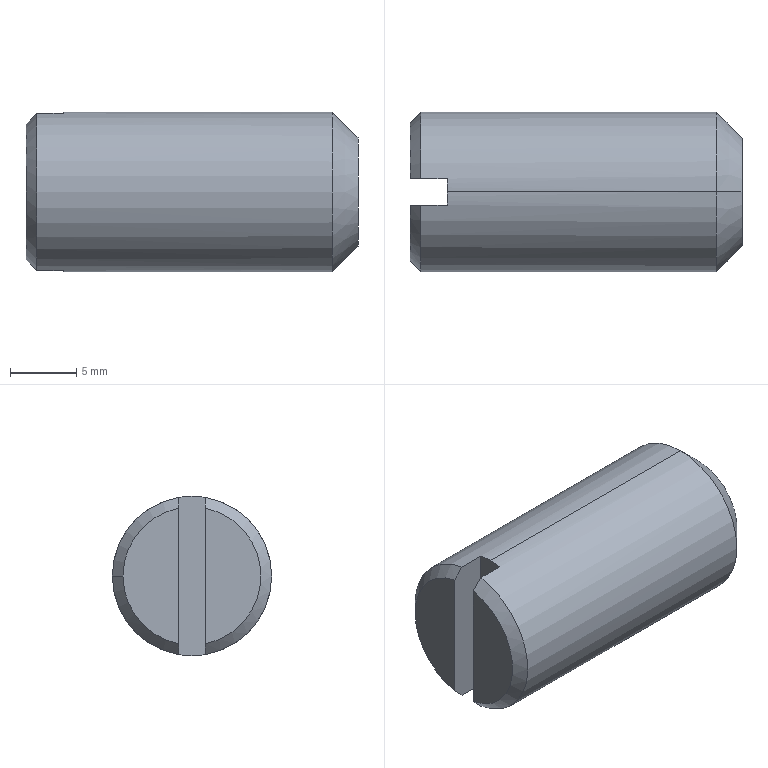Part | STEP file | 1 solid | 13 faces | box 25 x 12 x 12 mm | volume 2688 mm3 | plane 6 | cone 5 | cylinder 2 | commonest cylinder face diameters 12 x2
STEP:
#1=CARTESIAN_POINT('',(0.,0.,0.));
#2=DIRECTION('',(0.,0.,1.));
#3=DIRECTION('',(1.,0.,0.));
#4=AXIS2_PLACEMENT_3D('',#1,#2,#3);
#5=CARTESIAN_POINT('',(0.,-1.,5.099));
#6=VERTEX_POINT('',#5);
#7=CARTESIAN_POINT('',(0.,-1.,-5.099));
#8=VERTEX_POINT('',#7);
#9=CARTESIAN_POINT('',(0.,-1.,-50.));
#10=DIRECTION('',(0.,0.,-1.));
#11=VECTOR('',#10,1.);
#12=LINE('',#9,#11);
#13=CARTESIAN_POINT('',(0.,5.196,0.));
#14=DIRECTION('',(1.,0.,0.));
#15=DIRECTION('',(0.,1.,0.));
#16=AXIS2_PLACEMENT_3D('',#13,#14,#15);
#17=PLANE('',#16);
#18=CARTESIAN_POINT('',(-6.196,-50.));
#19=DIRECTION('',(0.,-1.));
#20=VECTOR('',#19,1.);
#21=LINE('',#18,#20);
#22=(GEOMETRIC_REPRESENTATION_CONTEXT(2)PARAMETRIC_REPRESENTATION_CONTEXT()REPRESENTATION_CONTEXT('',''));
#23=DEFINITIONAL_REPRESENTATION('',(#21),#22);
#24=PCURVE('',#17,#23);
#25=CARTESIAN_POINT('',(0.,-1.,-50.));
#26=DIRECTION('',(0.,-1.,0.));
#27=DIRECTION('',(0.,0.,-1.));
#28=AXIS2_PLACEMENT_3D('',#25,#26,#27);
#29=PLANE('',#28);
#30=CARTESIAN_POINT('',(0.,0.));
#31=DIRECTION('',(1.,0.));
#32=VECTOR('',#31,1.);
#33=LINE('',#30,#32);
#34=(GEOMETRIC_REPRESENTATION_CONTEXT(2)PARAMETRIC_REPRESENTATION_CONTEXT()REPRESENTATION_CONTEXT('',''));
#35=DEFINITIONAL_REPRESENTATION('',(#33),#34);
#36=PCURVE('',#29,#35);
#37=SURFACE_CURVE('',#12,(#24,#36),.PCURVE_S1.);
#38=EDGE_CURVE('',#6,#8,#37,.T.);
#39=ORIENTED_EDGE('',*,*,#38,.T.);
#40=CARTESIAN_POINT('',(0.,0.,0.));
#41=DIRECTION('',(1.,0.,0.));
#42=DIRECTION('',(0.,1.,0.));
#43=AXIS2_PLACEMENT_3D('',#40,#41,#42);
#44=CIRCLE('',#43,5.196);
#45=CARTESIAN_POINT('',(-5.196,0.));
#46=DIRECTION('',(1.,0.));
#47=AXIS2_PLACEMENT_2D('',#45,#46);
#48=CIRCLE('',#47,5.196);
#49=(GEOMETRIC_REPRESENTATION_CONTEXT(2)PARAMETRIC_REPRESENTATION_CONTEXT()REPRESENTATION_CONTEXT('',''));
#50=DEFINITIONAL_REPRESENTATION('',(#48),#49);
#51=PCURVE('',#17,#50);
#52=CARTESIAN_POINT('',(0.804,0.,0.));
#53=DIRECTION('',(1.,0.,0.));
#54=DIRECTION('',(0.,1.,0.));
#55=AXIS2_PLACEMENT_3D('',#52,#53,#54);
#56=CONICAL_SURFACE('',#55,6.,0.7854);
#57=CARTESIAN_POINT('',(0.,-0.804));
#58=DIRECTION('',(1.,0.));
#59=VECTOR('',#58,1.);
#60=LINE('',#57,#59);
#61=(GEOMETRIC_REPRESENTATION_CONTEXT(2)PARAMETRIC_REPRESENTATION_CONTEXT()REPRESENTATION_CONTEXT('',''));
#62=DEFINITIONAL_REPRESENTATION('',(#60),#61);
#63=PCURVE('',#56,#62);
#64=SURFACE_CURVE('',#44,(#51,#63),.PCURVE_S1.);
#65=EDGE_CURVE('',#6,#8,#64,.T.);
#66=ORIENTED_EDGE('',*,*,#65,.F.);
#67=EDGE_LOOP('',(#39,#66));
#68=FACE_BOUND('',#67,.T.);
#69=ADVANCED_FACE('',(#68),#17,.F.);
#70=CARTESIAN_POINT('',(25.,0.,4.07));
#71=VERTEX_POINT('',#70);
#72=CARTESIAN_POINT('',(25.,0.,-4.07));
#73=VERTEX_POINT('',#72);
#74=CARTESIAN_POINT('',(25.,0.,0.));
#75=DIRECTION('',(-1.,0.,0.));
#76=DIRECTION('',(0.,0.,1.));
#77=AXIS2_PLACEMENT_3D('',#74,#75,#76);
#78=CIRCLE('',#77,4.07);
#79=CARTESIAN_POINT('',(25.,0.,0.));
#80=DIRECTION('',(-1.,0.,0.));
#81=DIRECTION('',(0.,0.,1.));
#82=AXIS2_PLACEMENT_3D('',#79,#80,#81);
#83=PLANE('',#82);
#84=CARTESIAN_POINT('',(0.,0.));
#85=DIRECTION('',(1.,0.));
#86=AXIS2_PLACEMENT_2D('',#84,#85);
#87=CIRCLE('',#86,4.07);
#88=(GEOMETRIC_REPRESENTATION_CONTEXT(2)PARAMETRIC_REPRESENTATION_CONTEXT()REPRESENTATION_CONTEXT('',''));
#89=DEFINITIONAL_REPRESENTATION('',(#87),#88);
#90=PCURVE('',#83,#89);
#91=CARTESIAN_POINT('',(23.07,0.,0.));
#92=DIRECTION('',(-1.,0.,0.));
#93=DIRECTION('',(0.,0.,1.));
#94=AXIS2_PLACEMENT_3D('',#91,#92,#93);
#95=CONICAL_SURFACE('',#94,6.,0.7854);
#96=CARTESIAN_POINT('',(0.,-1.93));
#97=DIRECTION('',(1.,0.));
#98=VECTOR('',#97,1.);
#99=LINE('',#96,#98);
#100=(GEOMETRIC_REPRESENTATION_CONTEXT(2)PARAMETRIC_REPRESENTATION_CONTEXT()REPRESENTATION_CONTEXT('',''));
#101=DEFINITIONAL_REPRESENTATION('',(#99),#100);
#102=PCURVE('',#95,#101);
#103=SURFACE_CURVE('',#78,(#90,#102),.PCURVE_S1.);
#104=EDGE_CURVE('',#71,#73,#103,.T.);
#105=ORIENTED_EDGE('',*,*,#104,.F.);
#106=CARTESIAN_POINT('',(25.,0.,0.));
#107=DIRECTION('',(-1.,0.,0.));
#108=DIRECTION('',(0.,0.,1.));
#109=AXIS2_PLACEMENT_3D('',#106,#107,#108);
#110=CIRCLE('',#109,4.07);
#111=CARTESIAN_POINT('',(0.,0.));
#112=DIRECTION('',(1.,0.));
#113=AXIS2_PLACEMENT_2D('',#111,#112);
#114=CIRCLE('',#113,4.07);
#115=(GEOMETRIC_REPRESENTATION_CONTEXT(2)PARAMETRIC_REPRESENTATION_CONTEXT()REPRESENTATION_CONTEXT('',''));
#116=DEFINITIONAL_REPRESENTATION('',(#114),#115);
#117=PCURVE('',#83,#116);
#118=CARTESIAN_POINT('',(23.07,0.,0.));
#119=DIRECTION('',(-1.,0.,0.));
#120=DIRECTION('',(0.,0.,1.));
#121=AXIS2_PLACEMENT_3D('',#118,#119,#120);
#122=CONICAL_SURFACE('',#121,6.,0.7854);
#123=CARTESIAN_POINT('',(0.,-1.93));
#124=DIRECTION('',(1.,0.));
#125=VECTOR('',#124,1.);
#126=LINE('',#123,#125);
#127=(GEOMETRIC_REPRESENTATION_CONTEXT(2)PARAMETRIC_REPRESENTATION_CONTEXT()REPRESENTATION_CONTEXT('',''));
#128=DEFINITIONAL_REPRESENTATION('',(#126),#127);
#129=PCURVE('',#122,#128);
#130=SURFACE_CURVE('',#110,(#117,#129),.PCURVE_S1.);
#131=EDGE_CURVE('',#73,#71,#130,.T.);
#132=ORIENTED_EDGE('',*,*,#131,.F.);
#133=EDGE_LOOP('',(#105,#132));
#134=FACE_BOUND('',#133,.T.);
#135=ADVANCED_FACE('',(#134),#83,.F.);
#136=CARTESIAN_POINT('',(0.,1.,-5.099));
#137=VERTEX_POINT('',#136);
#138=CARTESIAN_POINT('',(0.,1.,5.099));
#139=VERTEX_POINT('',#138);
#140=CARTESIAN_POINT('',(0.,1.,-50.));
#141=DIRECTION('',(0.,0.,1.));
#142=VECTOR('',#141,1.);
#143=LINE('',#140,#142);
#144=CARTESIAN_POINT('',(0.,5.196,0.));
#145=DIRECTION('',(1.,0.,0.));
#146=DIRECTION('',(0.,1.,0.));
#147=AXIS2_PLACEMENT_3D('',#144,#145,#146);
#148=PLANE('',#147);
#149=CARTESIAN_POINT('',(-4.196,-50.));
#150=DIRECTION('',(0.,1.));
#151=VECTOR('',#150,1.);
#152=LINE('',#149,#151);
#153=(GEOMETRIC_REPRESENTATION_CONTEXT(2)PARAMETRIC_REPRESENTATION_CONTEXT()REPRESENTATION_CONTEXT('',''));
#154=DEFINITIONAL_REPRESENTATION('',(#152),#153);
#155=PCURVE('',#148,#154);
#156=CARTESIAN_POINT('',(0.,1.,-50.));
#157=DIRECTION('',(0.,1.,0.));
#158=DIRECTION('',(1.,0.,0.));
#159=AXIS2_PLACEMENT_3D('',#156,#157,#158);
#160=PLANE('',#159);
#161=CARTESIAN_POINT('',(0.,0.));
#162=DIRECTION('',(0.,-1.));
#163=VECTOR('',#162,1.);
#164=LINE('',#161,#163);
#165=(GEOMETRIC_REPRESENTATION_CONTEXT(2)PARAMETRIC_REPRESENTATION_CONTEXT()REPRESENTATION_CONTEXT('',''));
#166=DEFINITIONAL_REPRESENTATION('',(#164),#165);
#167=PCURVE('',#160,#166);
#168=SURFACE_CURVE('',#143,(#155,#167),.PCURVE_S1.);
#169=EDGE_CURVE('',#137,#139,#168,.T.);
#170=ORIENTED_EDGE('',*,*,#169,.T.);
#171=CARTESIAN_POINT('',(0.,5.196,0.));
#172=VERTEX_POINT('',#171);
#173=CARTESIAN_POINT('',(0.,0.,0.));
#174=DIRECTION('',(1.,0.,0.));
#175=DIRECTION('',(0.,1.,0.));
#176=AXIS2_PLACEMENT_3D('',#173,#174,#175);
#177=CIRCLE('',#176,5.196);
#178=CARTESIAN_POINT('',(-5.196,0.));
#179=DIRECTION('',(1.,0.));
#180=AXIS2_PLACEMENT_2D('',#178,#179);
#181=CIRCLE('',#180,5.196);
#182=(GEOMETRIC_REPRESENTATION_CONTEXT(2)PARAMETRIC_REPRESENTATION_CONTEXT()REPRESENTATION_CONTEXT('',''));
#183=DEFINITIONAL_REPRESENTATION('',(#181),#182);
#184=PCURVE('',#148,#183);
#185=CARTESIAN_POINT('',(0.804,0.,0.));
#186=DIRECTION('',(1.,0.,0.));
#187=DIRECTION('',(0.,1.,0.));
#188=AXIS2_PLACEMENT_3D('',#185,#186,#187);
#189=CONICAL_SURFACE('',#188,6.,0.7854);
#190=CARTESIAN_POINT('',(0.,-0.804));
#191=DIRECTION('',(1.,0.));
#192=VECTOR('',#191,1.);
#193=LINE('',#190,#192);
#194=(GEOMETRIC_REPRESENTATION_CONTEXT(2)PARAMETRIC_REPRESENTATION_CONTEXT()REPRESENTATION_CONTEXT('',''));
#195=DEFINITIONAL_REPRESENTATION('',(#193),#194);
#196=PCURVE('',#189,#195);
#197=SURFACE_CURVE('',#177,(#184,#196),.PCURVE_S1.);
#198=EDGE_CURVE('',#172,#139,#197,.T.);
#199=ORIENTED_EDGE('',*,*,#198,.F.);
#200=CARTESIAN_POINT('',(0.,0.,0.));
#201=DIRECTION('',(1.,0.,0.));
#202=DIRECTION('',(0.,1.,0.));
#203=AXIS2_PLACEMENT_3D('',#200,#201,#202);
#204=CIRCLE('',#203,5.196);
#205=CARTESIAN_POINT('',(-5.196,0.));
#206=DIRECTION('',(1.,0.));
#207=AXIS2_PLACEMENT_2D('',#205,#206);
#208=CIRCLE('',#207,5.196);
#209=(GEOMETRIC_REPRESENTATION_CONTEXT(2)PARAMETRIC_REPRESENTATION_CONTEXT()REPRESENTATION_CONTEXT('',''));
#210=DEFINITIONAL_REPRESENTATION('',(#208),#209);
#211=PCURVE('',#148,#210);
#212=CARTESIAN_POINT('',(0.804,0.,0.));
#213=DIRECTION('',(1.,0.,0.));
#214=DIRECTION('',(0.,1.,0.));
#215=AXIS2_PLACEMENT_3D('',#212,#213,#214);
#216=CONICAL_SURFACE('',#215,6.,0.7854);
#217=CARTESIAN_POINT('',(0.,-0.804));
#218=DIRECTION('',(1.,0.));
#219=VECTOR('',#218,1.);
#220=LINE('',#217,#219);
#221=(GEOMETRIC_REPRESENTATION_CONTEXT(2)PARAMETRIC_REPRESENTATION_CONTEXT()REPRESENTATION_CONTEXT('',''));
#222=DEFINITIONAL_REPRESENTATION('',(#220),#221);
#223=PCURVE('',#216,#222);
#224=SURFACE_CURVE('',#204,(#211,#223),.PCURVE_S1.);
#225=EDGE_CURVE('',#137,#172,#224,.T.);
#226=ORIENTED_EDGE('',*,*,#225,.F.);
#227=EDGE_LOOP('',(#170,#199,#226));
#228=FACE_BOUND('',#227,.T.);
#229=ADVANCED_FACE('',(#228),#148,.F.);
#230=CARTESIAN_POINT('',(2.8,-1.,-5.916));
#231=VERTEX_POINT('',#230);
#232=CARTESIAN_POINT('',(2.8,0.,-6.));
#233=VERTEX_POINT('',#232);
#234=CARTESIAN_POINT('',(2.8,0.,0.));
#235=DIRECTION('',(1.,0.,0.));
#236=DIRECTION('',(0.,0.,1.));
#237=AXIS2_PLACEMENT_3D('',#234,#235,#236);
#238=CIRCLE('',#237,6.);
#239=CARTESIAN_POINT('',(2.8,-1.,-50.));
#240=DIRECTION('',(1.,0.,0.));
#241=DIRECTION('',(0.,1.,0.));
#242=AXIS2_PLACEMENT_3D('',#239,#240,#241);
#243=PLANE('',#242);
#244=CARTESIAN_POINT('',(1.,50.));
#245=DIRECTION('',(0.,1.));
#246=AXIS2_PLACEMENT_2D('',#244,#245);
#247=CIRCLE('',#246,6.);
#248=(GEOMETRIC_REPRESENTATION_CONTEXT(2)PARAMETRIC_REPRESENTATION_CONTEXT()REPRESENTATION_CONTEXT('',''));
#249=DEFINITIONAL_REPRESENTATION('',(#247),#248);
#250=PCURVE('',#243,#249);
#251=CARTESIAN_POINT('',(-0.5499,0.,0.));
#252=DIRECTION('',(-1.,0.,0.));
#253=DIRECTION('',(0.,0.,1.));
#254=AXIS2_PLACEMENT_3D('',#251,#252,#253);
#255=CYLINDRICAL_SURFACE('',#254,6.);
#256=CARTESIAN_POINT('',(6.283,-3.35));
#257=DIRECTION('',(-1.,0.));
#258=VECTOR('',#257,1.);
#259=LINE('',#256,#258);
#260=(GEOMETRIC_REPRESENTATION_CONTEXT(2)PARAMETRIC_REPRESENTATION_CONTEXT()REPRESENTATION_CONTEXT('',''));
#261=DEFINITIONAL_REPRESENTATION('',(#259),#260);
#262=PCURVE('',#255,#261);
#263=SURFACE_CURVE('',#238,(#250,#262),.PCURVE_S1.);
#264=EDGE_CURVE('',#231,#233,#263,.T.);
#265=ORIENTED_EDGE('',*,*,#264,.F.);
#266=CARTESIAN_POINT('',(2.8,-1.,5.916));
#267=VERTEX_POINT('',#266);
#268=CARTESIAN_POINT('',(2.8,-1.,-50.));
#269=DIRECTION('',(0.,0.,1.));
#270=VECTOR('',#269,1.);
#271=LINE('',#268,#270);
#272=CARTESIAN_POINT('',(0.,0.));
#273=DIRECTION('',(0.,1.));
#274=VECTOR('',#273,1.);
#275=LINE('',#272,#274);
#276=(GEOMETRIC_REPRESENTATION_CONTEXT(2)PARAMETRIC_REPRESENTATION_CONTEXT()REPRESENTATION_CONTEXT('',''));
#277=DEFINITIONAL_REPRESENTATION('',(#275),#276);
#278=PCURVE('',#243,#277);
#279=CARTESIAN_POINT('',(0.,2.8));
#280=DIRECTION('',(-1.,0.));
#281=VECTOR('',#280,1.);
#282=LINE('',#279,#281);
#283=(GEOMETRIC_REPRESENTATION_CONTEXT(2)PARAMETRIC_REPRESENTATION_CONTEXT()REPRESENTATION_CONTEXT('',''));
#284=DEFINITIONAL_REPRESENTATION('',(#282),#283);
#285=PCURVE('',#29,#284);
#286=SURFACE_CURVE('',#271,(#278,#285),.PCURVE_S1.);
#287=EDGE_CURVE('',#231,#267,#286,.T.);
#288=ORIENTED_EDGE('',*,*,#287,.T.);
#289=CARTESIAN_POINT('',(2.8,0.,6.));
#290=VERTEX_POINT('',#289);
#291=CARTESIAN_POINT('',(2.8,0.,0.));
#292=DIRECTION('',(1.,0.,0.));
#293=DIRECTION('',(0.,0.,1.));
#294=AXIS2_PLACEMENT_3D('',#291,#292,#293);
#295=CIRCLE('',#294,6.);
#296=CARTESIAN_POINT('',(1.,50.));
#297=DIRECTION('',(0.,1.));
#298=AXIS2_PLACEMENT_2D('',#296,#297);
#299=CIRCLE('',#298,6.);
#300=(GEOMETRIC_REPRESENTATION_CONTEXT(2)PARAMETRIC_REPRESENTATION_CONTEXT()REPRESENTATION_CONTEXT('',''));
#301=DEFINITIONAL_REPRESENTATION('',(#299),#300);
#302=PCURVE('',#243,#301);
#303=CARTESIAN_POINT('',(6.283,-3.35));
#304=DIRECTION('',(-1.,0.));
#305=VECTOR('',#304,1.);
#306=LINE('',#303,#305);
#307=(GEOMETRIC_REPRESENTATION_CONTEXT(2)PARAMETRIC_REPRESENTATION_CONTEXT()REPRESENTATION_CONTEXT('',''));
#308=DEFINITIONAL_REPRESENTATION('',(#306),#307);
#309=PCURVE('',#255,#308);
#310=SURFACE_CURVE('',#295,(#302,#309),.PCURVE_S1.);
#311=EDGE_CURVE('',#290,#267,#310,.T.);
#312=ORIENTED_EDGE('',*,*,#311,.F.);
#313=CARTESIAN_POINT('',(2.8,1.,5.916));
#314=VERTEX_POINT('',#313);
#315=CARTESIAN_POINT('',(2.8,0.,0.));
#316=DIRECTION('',(1.,0.,0.));
#317=DIRECTION('',(0.,0.,1.));
#318=AXIS2_PLACEMENT_3D('',#315,#316,#317);
#319=CIRCLE('',#318,6.);
#320=CARTESIAN_POINT('',(1.,50.));
#321=DIRECTION('',(0.,1.));
#322=AXIS2_PLACEMENT_2D('',#320,#321);
#323=CIRCLE('',#322,6.);
#324=(GEOMETRIC_REPRESENTATION_CONTEXT(2)PARAMETRIC_REPRESENTATION_CONTEXT()REPRESENTATION_CONTEXT('',''));
#325=DEFINITIONAL_REPRESENTATION('',(#323),#324);
#326=PCURVE('',#243,#325);
#327=CARTESIAN_POINT('',(-0.5499,0.,0.));
#328=DIRECTION('',(-1.,0.,0.));
#329=DIRECTION('',(0.,0.,1.));
#330=AXIS2_PLACEMENT_3D('',#327,#328,#329);
#331=CYLINDRICAL_SURFACE('',#330,6.);
#332=CARTESIAN_POINT('',(6.283,-3.35));
#333=DIRECTION('',(-1.,0.));
#334=VECTOR('',#333,1.);
#335=LINE('',#332,#334);
#336=(GEOMETRIC_REPRESENTATION_CONTEXT(2)PARAMETRIC_REPRESENTATION_CONTEXT()REPRESENTATION_CONTEXT('',''));
#337=DEFINITIONAL_REPRESENTATION('',(#335),#336);
#338=PCURVE('',#331,#337);
#339=SURFACE_CURVE('',#319,(#326,#338),.PCURVE_S1.);
#340=EDGE_CURVE('',#314,#290,#339,.T.);
#341=ORIENTED_EDGE('',*,*,#340,.F.);
#342=CARTESIAN_POINT('',(2.8,1.,-5.916));
#343=VERTEX_POINT('',#342);
#344=CARTESIAN_POINT('',(2.8,1.,-50.));
#345=DIRECTION('',(0.,0.,-1.));
#346=VECTOR('',#345,1.);
#347=LINE('',#344,#346);
#348=CARTESIAN_POINT('',(2.,0.));
#349=DIRECTION('',(0.,-1.));
#350=VECTOR('',#349,1.);
#351=LINE('',#348,#350);
#352=(GEOMETRIC_REPRESENTATION_CONTEXT(2)PARAMETRIC_REPRESENTATION_CONTEXT()REPRESENTATION_CONTEXT('',''));
#353=DEFINITIONAL_REPRESENTATION('',(#351),#352);
#354=PCURVE('',#243,#353);
#355=CARTESIAN_POINT('',(2.8,0.));
#356=DIRECTION('',(0.,1.));
#357=VECTOR('',#356,1.);
#358=LINE('',#355,#357);
#359=(GEOMETRIC_REPRESENTATION_CONTEXT(2)PARAMETRIC_REPRESENTATION_CONTEXT()REPRESENTATION_CONTEXT('',''));
#360=DEFINITIONAL_REPRESENTATION('',(#358),#359);
#361=PCURVE('',#160,#360);
#362=SURFACE_CURVE('',#347,(#354,#361),.PCURVE_S1.);
#363=EDGE_CURVE('',#314,#343,#362,.T.);
#364=ORIENTED_EDGE('',*,*,#363,.T.);
#365=CARTESIAN_POINT('',(2.8,0.,0.));
#366=DIRECTION('',(1.,0.,0.));
#367=DIRECTION('',(0.,0.,1.));
#368=AXIS2_PLACEMENT_3D('',#365,#366,#367);
#369=CIRCLE('',#368,6.);
#370=CARTESIAN_POINT('',(1.,50.));
#371=DIRECTION('',(0.,1.));
#372=AXIS2_PLACEMENT_2D('',#370,#371);
#373=CIRCLE('',#372,6.);
#374=(GEOMETRIC_REPRESENTATION_CONTEXT(2)PARAMETRIC_REPRESENTATION_CONTEXT()REPRESENTATION_CONTEXT('',''));
#375=DEFINITIONAL_REPRESENTATION('',(#373),#374);
#376=PCURVE('',#243,#375);
#377=CARTESIAN_POINT('',(6.283,-3.35));
#378=DIRECTION('',(-1.,0.));
#379=VECTOR('',#378,1.);
#380=LINE('',#377,#379);
#381=(GEOMETRIC_REPRESENTATION_CONTEXT(2)PARAMETRIC_REPRESENTATION_CONTEXT()REPRESENTATION_CONTEXT('',''));
#382=DEFINITIONAL_REPRESENTATION('',(#380),#381);
#383=PCURVE('',#331,#382);
#384=SURFACE_CURVE('',#369,(#376,#383),.PCURVE_S1.);
#385=EDGE_CURVE('',#233,#343,#384,.T.);
#386=ORIENTED_EDGE('',*,*,#385,.F.);
#387=EDGE_LOOP('',(#265,#288,#312,#341,#364,#386));
#388=FACE_BOUND('',#387,.T.);
#389=ADVANCED_FACE('',(#388),#243,.F.);
#390=ORIENTED_EDGE('',*,*,#65,.T.);
#391=CARTESIAN_POINT('',(0.804,-1.,-5.916));
#392=VERTEX_POINT('',#391);
#393=CARTESIAN_POINT('',(0.,-1.,-5.099));
#394=CARTESIAN_POINT('',(0.2677,-1.,-5.372));
#395=CARTESIAN_POINT('',(0.5357,-1.,-5.644));
#396=CARTESIAN_POINT('',(0.804,-1.,-5.916));
#397=B_SPLINE_CURVE_WITH_KNOTS('',3,(#393,#394,#395,#396),.UNSPECIFIED.,.F.,.F.,(4,4),(0.,0.001146),.PIECEWISE_BEZIER_KNOTS.);
#398=CARTESIAN_POINT('',(4.519,-0.804));
#399=CARTESIAN_POINT('',(4.519,-0.7918));
#400=CARTESIAN_POINT('',(4.52,-0.7675));
#401=CARTESIAN_POINT('',(4.521,-0.731));
#402=CARTESIAN_POINT('',(4.523,-0.6945));
#403=CARTESIAN_POINT('',(4.524,-0.658));
#404=CARTESIAN_POINT('',(4.525,-0.6215));
#405=CARTESIAN_POINT('',(4.527,-0.5849));
#406=CARTESIAN_POINT('',(4.528,-0.5484));
#407=CARTESIAN_POINT('',(4.529,-0.5119));
#408=CARTESIAN_POINT('',(4.53,-0.4753));
#409=CARTESIAN_POINT('',(4.532,-0.4388));
#410=CARTESIAN_POINT('',(4.533,-0.4022));
#411=CARTESIAN_POINT('',(4.534,-0.3657));
#412=CARTESIAN_POINT('',(4.535,-0.3291));
#413=CARTESIAN_POINT('',(4.536,-0.2926));
#414=CARTESIAN_POINT('',(4.537,-0.256));
#415=CARTESIAN_POINT('',(4.539,-0.2195));
#416=CARTESIAN_POINT('',(4.54,-0.1829));
#417=CARTESIAN_POINT('',(4.541,-0.1463));
#418=CARTESIAN_POINT('',(4.542,-0.1097));
#419=CARTESIAN_POINT('',(4.543,-0.07317));
#420=CARTESIAN_POINT('',(4.544,-0.03659));
#421=CARTESIAN_POINT('',(4.545,-0.0122));
#422=CARTESIAN_POINT('',(4.545,0.));
#423=B_SPLINE_CURVE_WITH_KNOTS('',3,(#398,#399,#400,#401,#402,#403,#404,#405,#406,#407,#408,#409,#410,#411,#412,#413,#414,#415,#416,#417,#418,#419,#420,#421,#422),.UNSPECIFIED.,.F.,.F.,(4,1,1,1,1,1,1,1,1,1,1,1,1,1,1,1,1,1,1,1,1,1,4),(0.,0.00005211,0.0001042,0.0001563,0.0002084,0.0002605,0.0003127,0.0003648,0.0004169,0.000469,0.0005211,0.0005732,0.0006253,0.0006774,0.0007295,0.0007816,0.0008338,0.0008859,0.000938,0.0009901,0.001042,0.001094,0.001146),.QUASI_UNIFORM_KNOTS.);
#424=(GEOMETRIC_REPRESENTATION_CONTEXT(2)PARAMETRIC_REPRESENTATION_CONTEXT()REPRESENTATION_CONTEXT('',''));
#425=DEFINITIONAL_REPRESENTATION('',(#423),#424);
#426=PCURVE('',#56,#425);
#427=CARTESIAN_POINT('',(-44.901,0.));
#428=CARTESIAN_POINT('',(-44.628,0.2677));
#429=CARTESIAN_POINT('',(-44.356,0.5357));
#430=CARTESIAN_POINT('',(-44.084,0.804));
#431=B_SPLINE_CURVE_WITH_KNOTS('',3,(#427,#428,#429,#430),.UNSPECIFIED.,.F.,.F.,(4,4),(0.,0.001146),.PIECEWISE_BEZIER_KNOTS.);
#432=(GEOMETRIC_REPRESENTATION_CONTEXT(2)PARAMETRIC_REPRESENTATION_CONTEXT()REPRESENTATION_CONTEXT('',''));
#433=DEFINITIONAL_REPRESENTATION('',(#431),#432);
#434=PCURVE('',#29,#433);
#435=SURFACE_CURVE('',#397,(#426,#434),.PCURVE_S1.);
#436=EDGE_CURVE('',#8,#392,#435,.T.);
#437=ORIENTED_EDGE('',*,*,#436,.T.);
#438=CARTESIAN_POINT('',(0.804,-1.,5.916));
#439=VERTEX_POINT('',#438);
#440=CARTESIAN_POINT('',(0.804,0.,0.));
#441=DIRECTION('',(1.,0.,0.));
#442=DIRECTION('',(0.,0.,1.));
#443=AXIS2_PLACEMENT_3D('',#440,#441,#442);
#444=CIRCLE('',#443,6.);
#445=CARTESIAN_POINT('',(1.571,0.));
#446=DIRECTION('',(1.,0.));
#447=VECTOR('',#446,1.);
#448=LINE('',#445,#447);
#449=(GEOMETRIC_REPRESENTATION_CONTEXT(2)PARAMETRIC_REPRESENTATION_CONTEXT()REPRESENTATION_CONTEXT('',''));
#450=DEFINITIONAL_REPRESENTATION('',(#448),#449);
#451=PCURVE('',#56,#450);
#452=CARTESIAN_POINT('',(6.283,-1.354));
#453=DIRECTION('',(-1.,0.));
#454=VECTOR('',#453,1.);
#455=LINE('',#452,#454);
#456=(GEOMETRIC_REPRESENTATION_CONTEXT(2)PARAMETRIC_REPRESENTATION_CONTEXT()REPRESENTATION_CONTEXT('',''));
#457=DEFINITIONAL_REPRESENTATION('',(#455),#456);
#458=PCURVE('',#255,#457);
#459=SURFACE_CURVE('',#444,(#451,#458),.PCURVE_S1.);
#460=EDGE_CURVE('',#439,#392,#459,.T.);
#461=ORIENTED_EDGE('',*,*,#460,.F.);
#462=CARTESIAN_POINT('',(0.804,-1.,5.916));
#463=CARTESIAN_POINT('',(0.5357,-1.,5.644));
#464=CARTESIAN_POINT('',(0.2677,-1.,5.372));
#465=CARTESIAN_POINT('',(0.,-1.,5.099));
#466=B_SPLINE_CURVE_WITH_KNOTS('',3,(#462,#463,#464,#465),.UNSPECIFIED.,.F.,.F.,(4,4),(0.,0.001146),.PIECEWISE_BEZIER_KNOTS.);
#467=CARTESIAN_POINT('',(1.738,0.));
#468=CARTESIAN_POINT('',(1.739,-0.0122));
#469=CARTESIAN_POINT('',(1.739,-0.03659));
#470=CARTESIAN_POINT('',(1.74,-0.07317));
#471=CARTESIAN_POINT('',(1.741,-0.1097));
#472=CARTESIAN_POINT('',(1.742,-0.1463));
#473=CARTESIAN_POINT('',(1.744,-0.1829));
#474=CARTESIAN_POINT('',(1.745,-0.2195));
#475=CARTESIAN_POINT('',(1.746,-0.256));
#476=CARTESIAN_POINT('',(1.747,-0.2926));
#477=CARTESIAN_POINT('',(1.748,-0.3291));
#478=CARTESIAN_POINT('',(1.749,-0.3657));
#479=CARTESIAN_POINT('',(1.75,-0.4022));
#480=CARTESIAN_POINT('',(1.752,-0.4388));
#481=CARTESIAN_POINT('',(1.753,-0.4753));
#482=CARTESIAN_POINT('',(1.754,-0.5119));
#483=CARTESIAN_POINT('',(1.755,-0.5484));
#484=CARTESIAN_POINT('',(1.757,-0.5849));
#485=CARTESIAN_POINT('',(1.758,-0.6215));
#486=CARTESIAN_POINT('',(1.759,-0.658));
#487=CARTESIAN_POINT('',(1.76,-0.6945));
#488=CARTESIAN_POINT('',(1.762,-0.731));
#489=CARTESIAN_POINT('',(1.763,-0.7675));
#490=CARTESIAN_POINT('',(1.764,-0.7918));
#491=CARTESIAN_POINT('',(1.764,-0.804));
#492=B_SPLINE_CURVE_WITH_KNOTS('',3,(#467,#468,#469,#470,#471,#472,#473,#474,#475,#476,#477,#478,#479,#480,#481,#482,#483,#484,#485,#486,#487,#488,#489,#490,#491),.UNSPECIFIED.,.F.,.F.,(4,1,1,1,1,1,1,1,1,1,1,1,1,1,1,1,1,1,1,1,1,1,4),(0.,0.00005211,0.0001042,0.0001563,0.0002084,0.0002605,0.0003127,0.0003648,0.0004169,0.000469,0.0005211,0.0005732,0.0006253,0.0006774,0.0007295,0.0007816,0.0008338,0.0008859,0.000938,0.0009901,0.001042,0.001094,0.001146),.QUASI_UNIFORM_KNOTS.);
#493=(GEOMETRIC_REPRESENTATION_CONTEXT(2)PARAMETRIC_REPRESENTATION_CONTEXT()REPRESENTATION_CONTEXT('',''));
#494=DEFINITIONAL_REPRESENTATION('',(#492),#493);
#495=PCURVE('',#56,#494);
#496=CARTESIAN_POINT('',(-55.916,0.804));
#497=CARTESIAN_POINT('',(-55.644,0.5357));
#498=CARTESIAN_POINT('',(-55.372,0.2677));
#499=CARTESIAN_POINT('',(-55.099,0.));
#500=B_SPLINE_CURVE_WITH_KNOTS('',3,(#496,#497,#498,#499),.UNSPECIFIED.,.F.,.F.,(4,4),(0.,0.001146),.PIECEWISE_BEZIER_KNOTS.);
#501=(GEOMETRIC_REPRESENTATION_CONTEXT(2)PARAMETRIC_REPRESENTATION_CONTEXT()REPRESENTATION_CONTEXT('',''));
#502=DEFINITIONAL_REPRESENTATION('',(#500),#501);
#503=PCURVE('',#29,#502);
#504=SURFACE_CURVE('',#466,(#495,#503),.PCURVE_S1.);
#505=EDGE_CURVE('',#439,#6,#504,.T.);
#506=ORIENTED_EDGE('',*,*,#505,.T.);
#507=EDGE_LOOP('',(#390,#437,#461,#506));
#508=FACE_BOUND('',#507,.T.);
#509=ADVANCED_FACE('',(#508),#56,.T.);
#510=CARTESIAN_POINT('',(-0.5499,-1.,-5.916));
#511=DIRECTION('',(1.,0.,0.));
#512=VECTOR('',#511,1.);
#513=LINE('',#510,#512);
#514=CARTESIAN_POINT('',(-44.084,-0.5499));
#515=DIRECTION('',(0.,1.));
#516=VECTOR('',#515,1.);
#517=LINE('',#514,#516);
#518=(GEOMETRIC_REPRESENTATION_CONTEXT(2)PARAMETRIC_REPRESENTATION_CONTEXT()REPRESENTATION_CONTEXT('',''));
#519=DEFINITIONAL_REPRESENTATION('',(#517),#518);
#520=PCURVE('',#29,#519);
#521=CARTESIAN_POINT('',(3.309,0.));
#522=DIRECTION('',(0.,-1.));
#523=VECTOR('',#522,1.);
#524=LINE('',#521,#523);
#525=(GEOMETRIC_REPRESENTATION_CONTEXT(2)PARAMETRIC_REPRESENTATION_CONTEXT()REPRESENTATION_CONTEXT('',''));
#526=DEFINITIONAL_REPRESENTATION('',(#524),#525);
#527=PCURVE('',#255,#526);
#528=SURFACE_CURVE('',#513,(#520,#527),.PCURVE_S1.);
#529=EDGE_CURVE('',#392,#231,#528,.T.);
#530=ORIENTED_EDGE('',*,*,#529,.F.);
#531=ORIENTED_EDGE('',*,*,#436,.F.);
#532=ORIENTED_EDGE('',*,*,#38,.F.);
#533=ORIENTED_EDGE('',*,*,#505,.F.);
#534=CARTESIAN_POINT('',(-0.5499,-1.,5.916));
#535=DIRECTION('',(-1.,0.,0.));
#536=VECTOR('',#535,1.);
#537=LINE('',#534,#536);
#538=CARTESIAN_POINT('',(-55.916,-0.5499));
#539=DIRECTION('',(0.,-1.));
#540=VECTOR('',#539,1.);
#541=LINE('',#538,#540);
#542=(GEOMETRIC_REPRESENTATION_CONTEXT(2)PARAMETRIC_REPRESENTATION_CONTEXT()REPRESENTATION_CONTEXT('',''));
#543=DEFINITIONAL_REPRESENTATION('',(#541),#542);
#544=PCURVE('',#29,#543);
#545=CARTESIAN_POINT('',(6.116,0.));
#546=DIRECTION('',(0.,1.));
#547=VECTOR('',#546,1.);
#548=LINE('',#545,#547);
#549=(GEOMETRIC_REPRESENTATION_CONTEXT(2)PARAMETRIC_REPRESENTATION_CONTEXT()REPRESENTATION_CONTEXT('',''));
#550=DEFINITIONAL_REPRESENTATION('',(#548),#549);
#551=PCURVE('',#255,#550);
#552=SURFACE_CURVE('',#537,(#544,#551),.PCURVE_S1.);
#553=EDGE_CURVE('',#267,#439,#552,.T.);
#554=ORIENTED_EDGE('',*,*,#553,.F.);
#555=ORIENTED_EDGE('',*,*,#287,.F.);
#556=EDGE_LOOP('',(#530,#531,#532,#533,#554,#555));
#557=FACE_BOUND('',#556,.T.);
#558=ADVANCED_FACE('',(#557),#29,.F.);
#559=CARTESIAN_POINT('',(23.07,0.,-6.));
#560=VERTEX_POINT('',#559);
#561=CARTESIAN_POINT('',(23.07,0.,-6.));
#562=DIRECTION('',(-0.7071,0.,-0.7071));
#563=VECTOR('',#562,1.);
#564=LINE('',#561,#563);
#565=CARTESIAN_POINT('',(3.142,0.));
#566=DIRECTION('',(0.,1.));
#567=VECTOR('',#566,1.);
#568=LINE('',#565,#567);
#569=(GEOMETRIC_REPRESENTATION_CONTEXT(2)PARAMETRIC_REPRESENTATION_CONTEXT()REPRESENTATION_CONTEXT('',''));
#570=DEFINITIONAL_REPRESENTATION('',(#568),#569);
#571=PCURVE('',#122,#570);
#572=CARTESIAN_POINT('',(3.142,0.));
#573=DIRECTION('',(0.,1.));
#574=VECTOR('',#573,1.);
#575=LINE('',#572,#574);
#576=(GEOMETRIC_REPRESENTATION_CONTEXT(2)PARAMETRIC_REPRESENTATION_CONTEXT()REPRESENTATION_CONTEXT('',''));
#577=DEFINITIONAL_REPRESENTATION('',(#575),#576);
#578=PCURVE('',#95,#577);
#579=SURFACE_CURVE('',#564,(#571,#578),.PCURVE_S1.);
#580=EDGE_CURVE('',#73,#560,#579,.T.);
#581=ORIENTED_EDGE('',*,*,#580,.F.);
#582=ORIENTED_EDGE('',*,*,#131,.T.);
#583=CARTESIAN_POINT('',(23.07,0.,6.));
#584=VERTEX_POINT('',#583);
#585=CARTESIAN_POINT('',(23.07,0.,6.));
#586=DIRECTION('',(-0.7071,0.,0.7071));
#587=VECTOR('',#586,1.);
#588=LINE('',#585,#587);
#589=CARTESIAN_POINT('',(6.283,0.));
#590=DIRECTION('',(0.,1.));
#591=VECTOR('',#590,1.);
#592=LINE('',#589,#591);
#593=(GEOMETRIC_REPRESENTATION_CONTEXT(2)PARAMETRIC_REPRESENTATION_CONTEXT()REPRESENTATION_CONTEXT('',''));
#594=DEFINITIONAL_REPRESENTATION('',(#592),#593);
#595=PCURVE('',#122,#594);
#596=CARTESIAN_POINT('',(0.,0.));
#597=DIRECTION('',(0.,1.));
#598=VECTOR('',#597,1.);
#599=LINE('',#596,#598);
#600=(GEOMETRIC_REPRESENTATION_CONTEXT(2)PARAMETRIC_REPRESENTATION_CONTEXT()REPRESENTATION_CONTEXT('',''));
#601=DEFINITIONAL_REPRESENTATION('',(#599),#600);
#602=PCURVE('',#95,#601);
#603=SURFACE_CURVE('',#588,(#595,#602),.PCURVE_S1.);
#604=EDGE_CURVE('',#71,#584,#603,.T.);
#605=ORIENTED_EDGE('',*,*,#604,.T.);
#606=CARTESIAN_POINT('',(23.07,0.,0.));
#607=DIRECTION('',(-1.,0.,0.));
#608=DIRECTION('',(0.,0.,1.));
#609=AXIS2_PLACEMENT_3D('',#606,#607,#608);
#610=CIRCLE('',#609,6.);
#611=CARTESIAN_POINT('',(0.,0.));
#612=DIRECTION('',(1.,0.));
#613=VECTOR('',#612,1.);
#614=LINE('',#611,#613);
#615=(GEOMETRIC_REPRESENTATION_CONTEXT(2)PARAMETRIC_REPRESENTATION_CONTEXT()REPRESENTATION_CONTEXT('',''));
#616=DEFINITIONAL_REPRESENTATION('',(#614),#615);
#617=PCURVE('',#122,#616);
#618=CARTESIAN_POINT('',(0.,-23.62));
#619=DIRECTION('',(1.,0.));
#620=VECTOR('',#619,1.);
#621=LINE('',#618,#620);
#622=(GEOMETRIC_REPRESENTATION_CONTEXT(2)PARAMETRIC_REPRESENTATION_CONTEXT()REPRESENTATION_CONTEXT('',''));
#623=DEFINITIONAL_REPRESENTATION('',(#621),#622);
#624=PCURVE('',#255,#623);
#625=SURFACE_CURVE('',#610,(#617,#624),.PCURVE_S1.);
#626=EDGE_CURVE('',#560,#584,#625,.T.);
#627=ORIENTED_EDGE('',*,*,#626,.F.);
#628=EDGE_LOOP('',(#581,#582,#605,#627));
#629=FACE_BOUND('',#628,.T.);
#630=ADVANCED_FACE('',(#629),#122,.T.);
#631=CARTESIAN_POINT('',(0.804,6.,0.));
#632=VERTEX_POINT('',#631);
#633=CARTESIAN_POINT('',(0.804,6.,0.));
#634=DIRECTION('',(0.7071,0.7071,0.));
#635=VECTOR('',#634,1.);
#636=LINE('',#633,#635);
#637=CARTESIAN_POINT('',(0.,0.));
#638=DIRECTION('',(0.,1.));
#639=VECTOR('',#638,1.);
#640=LINE('',#637,#639);
#641=(GEOMETRIC_REPRESENTATION_CONTEXT(2)PARAMETRIC_REPRESENTATION_CONTEXT()REPRESENTATION_CONTEXT('',''));
#642=DEFINITIONAL_REPRESENTATION('',(#640),#641);
#643=PCURVE('',#189,#642);
#644=CARTESIAN_POINT('',(6.283,0.));
#645=DIRECTION('',(0.,1.));
#646=VECTOR('',#645,1.);
#647=LINE('',#644,#646);
#648=(GEOMETRIC_REPRESENTATION_CONTEXT(2)PARAMETRIC_REPRESENTATION_CONTEXT()REPRESENTATION_CONTEXT('',''));
#649=DEFINITIONAL_REPRESENTATION('',(#647),#648);
#650=PCURVE('',#216,#649);
#651=SURFACE_CURVE('',#636,(#643,#650),.PCURVE_S1.);
#652=EDGE_CURVE('',#172,#632,#651,.T.);
#653=ORIENTED_EDGE('',*,*,#652,.F.);
#654=ORIENTED_EDGE('',*,*,#198,.T.);
#655=CARTESIAN_POINT('',(0.804,1.,5.916));
#656=VERTEX_POINT('',#655);
#657=CARTESIAN_POINT('',(0.,1.,5.099));
#658=CARTESIAN_POINT('',(0.2677,1.,5.372));
#659=CARTESIAN_POINT('',(0.5357,1.,5.644));
#660=CARTESIAN_POINT('',(0.804,1.,5.916));
#661=B_SPLINE_CURVE_WITH_KNOTS('',3,(#657,#658,#659,#660),.UNSPECIFIED.,.F.,.F.,(4,4),(0.,0.001146),.PIECEWISE_BEZIER_KNOTS.);
#662=CARTESIAN_POINT('',(1.377,-0.804));
#663=CARTESIAN_POINT('',(1.378,-0.7918));
#664=CARTESIAN_POINT('',(1.379,-0.7675));
#665=CARTESIAN_POINT('',(1.38,-0.731));
#666=CARTESIAN_POINT('',(1.381,-0.6945));
#667=CARTESIAN_POINT('',(1.382,-0.658));
#668=CARTESIAN_POINT('',(1.384,-0.6215));
#669=CARTESIAN_POINT('',(1.385,-0.5849));
#670=CARTESIAN_POINT('',(1.386,-0.5484));
#671=CARTESIAN_POINT('',(1.388,-0.5119));
#672=CARTESIAN_POINT('',(1.389,-0.4753));
#673=CARTESIAN_POINT('',(1.39,-0.4388));
#674=CARTESIAN_POINT('',(1.391,-0.4022));
#675=CARTESIAN_POINT('',(1.392,-0.3657));
#676=CARTESIAN_POINT('',(1.394,-0.3291));
#677=CARTESIAN_POINT('',(1.395,-0.2926));
#678=CARTESIAN_POINT('',(1.396,-0.256));
#679=CARTESIAN_POINT('',(1.397,-0.2195));
#680=CARTESIAN_POINT('',(1.398,-0.1829));
#681=CARTESIAN_POINT('',(1.399,-0.1463));
#682=CARTESIAN_POINT('',(1.4,-0.1097));
#683=CARTESIAN_POINT('',(1.401,-0.07317));
#684=CARTESIAN_POINT('',(1.402,-0.03659));
#685=CARTESIAN_POINT('',(1.403,-0.0122));
#686=CARTESIAN_POINT('',(1.403,0.));
#687=B_SPLINE_CURVE_WITH_KNOTS('',3,(#662,#663,#664,#665,#666,#667,#668,#669,#670,#671,#672,#673,#674,#675,#676,#677,#678,#679,#680,#681,#682,#683,#684,#685,#686),.UNSPECIFIED.,.F.,.F.,(4,1,1,1,1,1,1,1,1,1,1,1,1,1,1,1,1,1,1,1,1,1,4),(0.,0.00005211,0.0001042,0.0001563,0.0002084,0.0002605,0.0003127,0.0003648,0.0004169,0.000469,0.0005211,0.0005732,0.0006253,0.0006774,0.0007295,0.0007816,0.0008338,0.0008859,0.000938,0.0009901,0.001042,0.001094,0.001146),.QUASI_UNIFORM_KNOTS.);
#688=(GEOMETRIC_REPRESENTATION_CONTEXT(2)PARAMETRIC_REPRESENTATION_CONTEXT()REPRESENTATION_CONTEXT('',''));
#689=DEFINITIONAL_REPRESENTATION('',(#687),#688);
#690=PCURVE('',#189,#689);
#691=CARTESIAN_POINT('',(0.,-55.099));
#692=CARTESIAN_POINT('',(0.2677,-55.372));
#693=CARTESIAN_POINT('',(0.5357,-55.644));
#694=CARTESIAN_POINT('',(0.804,-55.916));
#695=B_SPLINE_CURVE_WITH_KNOTS('',3,(#691,#692,#693,#694),.UNSPECIFIED.,.F.,.F.,(4,4),(0.,0.001146),.PIECEWISE_BEZIER_KNOTS.);
#696=(GEOMETRIC_REPRESENTATION_CONTEXT(2)PARAMETRIC_REPRESENTATION_CONTEXT()REPRESENTATION_CONTEXT('',''));
#697=DEFINITIONAL_REPRESENTATION('',(#695),#696);
#698=PCURVE('',#160,#697);
#699=SURFACE_CURVE('',#661,(#690,#698),.PCURVE_S1.);
#700=EDGE_CURVE('',#139,#656,#699,.T.);
#701=ORIENTED_EDGE('',*,*,#700,.T.);
#702=CARTESIAN_POINT('',(0.804,0.,0.));
#703=DIRECTION('',(1.,0.,0.));
#704=DIRECTION('',(0.,0.,1.));
#705=AXIS2_PLACEMENT_3D('',#702,#703,#704);
#706=CIRCLE('',#705,6.);
#707=CARTESIAN_POINT('',(-4.712,0.));
#708=DIRECTION('',(1.,0.));
#709=VECTOR('',#708,1.);
#710=LINE('',#707,#709);
#711=(GEOMETRIC_REPRESENTATION_CONTEXT(2)PARAMETRIC_REPRESENTATION_CONTEXT()REPRESENTATION_CONTEXT('',''));
#712=DEFINITIONAL_REPRESENTATION('',(#710),#711);
#713=PCURVE('',#189,#712);
#714=CARTESIAN_POINT('',(6.283,-1.354));
#715=DIRECTION('',(-1.,0.));
#716=VECTOR('',#715,1.);
#717=LINE('',#714,#716);
#718=(GEOMETRIC_REPRESENTATION_CONTEXT(2)PARAMETRIC_REPRESENTATION_CONTEXT()REPRESENTATION_CONTEXT('',''));
#719=DEFINITIONAL_REPRESENTATION('',(#717),#718);
#720=PCURVE('',#331,#719);
#721=SURFACE_CURVE('',#706,(#713,#720),.PCURVE_S1.);
#722=EDGE_CURVE('',#632,#656,#721,.T.);
#723=ORIENTED_EDGE('',*,*,#722,.F.);
#724=EDGE_LOOP('',(#653,#654,#701,#723));
#725=FACE_BOUND('',#724,.T.);
#726=ADVANCED_FACE('',(#725),#189,.T.);
#727=CARTESIAN_POINT('',(-0.5499,1.,5.916));
#728=DIRECTION('',(1.,0.,0.));
#729=VECTOR('',#728,1.);
#730=LINE('',#727,#729);
#731=CARTESIAN_POINT('',(-0.5499,-55.916));
#732=DIRECTION('',(1.,0.));
#733=VECTOR('',#732,1.);
#734=LINE('',#731,#733);
#735=(GEOMETRIC_REPRESENTATION_CONTEXT(2)PARAMETRIC_REPRESENTATION_CONTEXT()REPRESENTATION_CONTEXT('',''));
#736=DEFINITIONAL_REPRESENTATION('',(#734),#735);
#737=PCURVE('',#160,#736);
#738=CARTESIAN_POINT('',(0.1674,0.));
#739=DIRECTION('',(0.,-1.));
#740=VECTOR('',#739,1.);
#741=LINE('',#738,#740);
#742=(GEOMETRIC_REPRESENTATION_CONTEXT(2)PARAMETRIC_REPRESENTATION_CONTEXT()REPRESENTATION_CONTEXT('',''));
#743=DEFINITIONAL_REPRESENTATION('',(#741),#742);
#744=PCURVE('',#331,#743);
#745=SURFACE_CURVE('',#730,(#737,#744),.PCURVE_S1.);
#746=EDGE_CURVE('',#656,#314,#745,.T.);
#747=ORIENTED_EDGE('',*,*,#746,.F.);
#748=ORIENTED_EDGE('',*,*,#700,.F.);
#749=ORIENTED_EDGE('',*,*,#169,.F.);
#750=CARTESIAN_POINT('',(0.804,1.,-5.916));
#751=VERTEX_POINT('',#750);
#752=CARTESIAN_POINT('',(0.804,1.,-5.916));
#753=CARTESIAN_POINT('',(0.5357,1.,-5.644));
#754=CARTESIAN_POINT('',(0.2677,1.,-5.372));
#755=CARTESIAN_POINT('',(0.,1.,-5.099));
#756=B_SPLINE_CURVE_WITH_KNOTS('',3,(#752,#753,#754,#755),.UNSPECIFIED.,.F.,.F.,(4,4),(0.,0.001146),.PIECEWISE_BEZIER_KNOTS.);
#757=CARTESIAN_POINT('',(0.804,-44.084));
#758=CARTESIAN_POINT('',(0.5357,-44.356));
#759=CARTESIAN_POINT('',(0.2677,-44.628));
#760=CARTESIAN_POINT('',(0.,-44.901));
#761=B_SPLINE_CURVE_WITH_KNOTS('',3,(#757,#758,#759,#760),.UNSPECIFIED.,.F.,.F.,(4,4),(0.,0.001146),.PIECEWISE_BEZIER_KNOTS.);
#762=(GEOMETRIC_REPRESENTATION_CONTEXT(2)PARAMETRIC_REPRESENTATION_CONTEXT()REPRESENTATION_CONTEXT('',''));
#763=DEFINITIONAL_REPRESENTATION('',(#761),#762);
#764=PCURVE('',#160,#763);
#765=CARTESIAN_POINT('',(4.88,0.));
#766=CARTESIAN_POINT('',(4.88,-0.0122));
#767=CARTESIAN_POINT('',(4.881,-0.03659));
#768=CARTESIAN_POINT('',(4.882,-0.07317));
#769=CARTESIAN_POINT('',(4.883,-0.1097));
#770=CARTESIAN_POINT('',(4.884,-0.1463));
#771=CARTESIAN_POINT('',(4.885,-0.1829));
#772=CARTESIAN_POINT('',(4.886,-0.2195));
#773=CARTESIAN_POINT('',(4.887,-0.256));
#774=CARTESIAN_POINT('',(4.889,-0.2926));
#775=CARTESIAN_POINT('',(4.89,-0.3291));
#776=CARTESIAN_POINT('',(4.891,-0.3657));
#777=CARTESIAN_POINT('',(4.892,-0.4022));
#778=CARTESIAN_POINT('',(4.893,-0.4388));
#779=CARTESIAN_POINT('',(4.894,-0.4753));
#780=CARTESIAN_POINT('',(4.896,-0.5119));
#781=CARTESIAN_POINT('',(4.897,-0.5484));
#782=CARTESIAN_POINT('',(4.898,-0.5849));
#783=CARTESIAN_POINT('',(4.899,-0.6215));
#784=CARTESIAN_POINT('',(4.901,-0.658));
#785=CARTESIAN_POINT('',(4.902,-0.6945));
#786=CARTESIAN_POINT('',(4.903,-0.731));
#787=CARTESIAN_POINT('',(4.905,-0.7675));
#788=CARTESIAN_POINT('',(4.906,-0.7918));
#789=CARTESIAN_POINT('',(4.906,-0.804));
#790=B_SPLINE_CURVE_WITH_KNOTS('',3,(#765,#766,#767,#768,#769,#770,#771,#772,#773,#774,#775,#776,#777,#778,#779,#780,#781,#782,#783,#784,#785,#786,#787,#788,#789),.UNSPECIFIED.,.F.,.F.,(4,1,1,1,1,1,1,1,1,1,1,1,1,1,1,1,1,1,1,1,1,1,4),(0.,0.00005211,0.0001042,0.0001563,0.0002084,0.0002605,0.0003127,0.0003648,0.0004169,0.000469,0.0005211,0.0005732,0.0006253,0.0006774,0.0007295,0.0007816,0.0008338,0.0008859,0.000938,0.0009901,0.001042,0.001094,0.001146),.QUASI_UNIFORM_KNOTS.);
#791=(GEOMETRIC_REPRESENTATION_CONTEXT(2)PARAMETRIC_REPRESENTATION_CONTEXT()REPRESENTATION_CONTEXT('',''));
#792=DEFINITIONAL_REPRESENTATION('',(#790),#791);
#793=PCURVE('',#216,#792);
#794=SURFACE_CURVE('',#756,(#764,#793),.PCURVE_S1.);
#795=EDGE_CURVE('',#751,#137,#794,.T.);
#796=ORIENTED_EDGE('',*,*,#795,.F.);
#797=CARTESIAN_POINT('',(-0.5499,1.,-5.916));
#798=DIRECTION('',(-1.,0.,0.));
#799=VECTOR('',#798,1.);
#800=LINE('',#797,#799);
#801=CARTESIAN_POINT('',(-0.5499,-44.084));
#802=DIRECTION('',(-1.,0.));
#803=VECTOR('',#802,1.);
#804=LINE('',#801,#803);
#805=(GEOMETRIC_REPRESENTATION_CONTEXT(2)PARAMETRIC_REPRESENTATION_CONTEXT()REPRESENTATION_CONTEXT('',''));
#806=DEFINITIONAL_REPRESENTATION('',(#804),#805);
#807=PCURVE('',#160,#806);
#808=CARTESIAN_POINT('',(2.974,0.));
#809=DIRECTION('',(0.,1.));
#810=VECTOR('',#809,1.);
#811=LINE('',#808,#810);
#812=(GEOMETRIC_REPRESENTATION_CONTEXT(2)PARAMETRIC_REPRESENTATION_CONTEXT()REPRESENTATION_CONTEXT('',''));
#813=DEFINITIONAL_REPRESENTATION('',(#811),#812);
#814=PCURVE('',#331,#813);
#815=SURFACE_CURVE('',#800,(#807,#814),.PCURVE_S1.);
#816=EDGE_CURVE('',#343,#751,#815,.T.);
#817=ORIENTED_EDGE('',*,*,#816,.F.);
#818=ORIENTED_EDGE('',*,*,#363,.F.);
#819=EDGE_LOOP('',(#747,#748,#749,#796,#817,#818));
#820=FACE_BOUND('',#819,.T.);
#821=ADVANCED_FACE('',(#820),#160,.F.);
#822=CARTESIAN_POINT('',(-0.5499,0.,-6.));
#823=DIRECTION('',(-1.,0.,0.));
#824=VECTOR('',#823,1.);
#825=LINE('',#822,#824);
#826=CARTESIAN_POINT('',(3.142,0.));
#827=DIRECTION('',(0.,1.));
#828=VECTOR('',#827,1.);
#829=LINE('',#826,#828);
#830=(GEOMETRIC_REPRESENTATION_CONTEXT(2)PARAMETRIC_REPRESENTATION_CONTEXT()REPRESENTATION_CONTEXT('',''));
#831=DEFINITIONAL_REPRESENTATION('',(#829),#830);
#832=PCURVE('',#255,#831);
#833=CARTESIAN_POINT('',(3.142,0.));
#834=DIRECTION('',(0.,1.));
#835=VECTOR('',#834,1.);
#836=LINE('',#833,#835);
#837=(GEOMETRIC_REPRESENTATION_CONTEXT(2)PARAMETRIC_REPRESENTATION_CONTEXT()REPRESENTATION_CONTEXT('',''));
#838=DEFINITIONAL_REPRESENTATION('',(#836),#837);
#839=PCURVE('',#331,#838);
#840=SURFACE_CURVE('',#825,(#832,#839),.PCURVE_S1.);
#841=EDGE_CURVE('',#560,#233,#840,.T.);
#842=ORIENTED_EDGE('',*,*,#841,.F.);
#843=ORIENTED_EDGE('',*,*,#626,.T.);
#844=CARTESIAN_POINT('',(-0.5499,0.,6.));
#845=DIRECTION('',(-1.,0.,0.));
#846=VECTOR('',#845,1.);
#847=LINE('',#844,#846);
#848=CARTESIAN_POINT('',(6.283,0.));
#849=DIRECTION('',(0.,1.));
#850=VECTOR('',#849,1.);
#851=LINE('',#848,#850);
#852=(GEOMETRIC_REPRESENTATION_CONTEXT(2)PARAMETRIC_REPRESENTATION_CONTEXT()REPRESENTATION_CONTEXT('',''));
#853=DEFINITIONAL_REPRESENTATION('',(#851),#852);
#854=PCURVE('',#255,#853);
#855=CARTESIAN_POINT('',(0.,0.));
#856=DIRECTION('',(0.,1.));
#857=VECTOR('',#856,1.);
#858=LINE('',#855,#857);
#859=(GEOMETRIC_REPRESENTATION_CONTEXT(2)PARAMETRIC_REPRESENTATION_CONTEXT()REPRESENTATION_CONTEXT('',''));
#860=DEFINITIONAL_REPRESENTATION('',(#858),#859);
#861=PCURVE('',#331,#860);
#862=SURFACE_CURVE('',#847,(#854,#861),.PCURVE_S1.);
#863=EDGE_CURVE('',#584,#290,#862,.T.);
#864=ORIENTED_EDGE('',*,*,#863,.T.);
#865=ORIENTED_EDGE('',*,*,#311,.T.);
#866=ORIENTED_EDGE('',*,*,#553,.T.);
#867=ORIENTED_EDGE('',*,*,#460,.T.);
#868=ORIENTED_EDGE('',*,*,#529,.T.);
#869=ORIENTED_EDGE('',*,*,#264,.T.);
#870=EDGE_LOOP('',(#842,#843,#864,#865,#866,#867,#868,#869));
#871=FACE_BOUND('',#870,.T.);
#872=ADVANCED_FACE('',(#871),#255,.T.);
#873=ORIENTED_EDGE('',*,*,#104,.T.);
#874=ORIENTED_EDGE('',*,*,#580,.T.);
#875=CARTESIAN_POINT('',(23.07,0.,0.));
#876=DIRECTION('',(-1.,0.,0.));
#877=DIRECTION('',(0.,0.,1.));
#878=AXIS2_PLACEMENT_3D('',#875,#876,#877);
#879=CIRCLE('',#878,6.);
#880=CARTESIAN_POINT('',(0.,0.));
#881=DIRECTION('',(1.,0.));
#882=VECTOR('',#881,1.);
#883=LINE('',#880,#882);
#884=(GEOMETRIC_REPRESENTATION_CONTEXT(2)PARAMETRIC_REPRESENTATION_CONTEXT()REPRESENTATION_CONTEXT('',''));
#885=DEFINITIONAL_REPRESENTATION('',(#883),#884);
#886=PCURVE('',#95,#885);
#887=CARTESIAN_POINT('',(0.,-23.62));
#888=DIRECTION('',(1.,0.));
#889=VECTOR('',#888,1.);
#890=LINE('',#887,#889);
#891=(GEOMETRIC_REPRESENTATION_CONTEXT(2)PARAMETRIC_REPRESENTATION_CONTEXT()REPRESENTATION_CONTEXT('',''));
#892=DEFINITIONAL_REPRESENTATION('',(#890),#891);
#893=PCURVE('',#331,#892);
#894=SURFACE_CURVE('',#879,(#886,#893),.PCURVE_S1.);
#895=EDGE_CURVE('',#584,#560,#894,.T.);
#896=ORIENTED_EDGE('',*,*,#895,.F.);
#897=ORIENTED_EDGE('',*,*,#604,.F.);
#898=EDGE_LOOP('',(#873,#874,#896,#897));
#899=FACE_BOUND('',#898,.T.);
#900=ADVANCED_FACE('',(#899),#95,.T.);
#901=ORIENTED_EDGE('',*,*,#225,.T.);
#902=ORIENTED_EDGE('',*,*,#652,.T.);
#903=CARTESIAN_POINT('',(0.804,0.,0.));
#904=DIRECTION('',(1.,0.,0.));
#905=DIRECTION('',(0.,0.,1.));
#906=AXIS2_PLACEMENT_3D('',#903,#904,#905);
#907=CIRCLE('',#906,6.);
#908=CARTESIAN_POINT('',(1.571,0.));
#909=DIRECTION('',(1.,0.));
#910=VECTOR('',#909,1.);
#911=LINE('',#908,#910);
#912=(GEOMETRIC_REPRESENTATION_CONTEXT(2)PARAMETRIC_REPRESENTATION_CONTEXT()REPRESENTATION_CONTEXT('',''));
#913=DEFINITIONAL_REPRESENTATION('',(#911),#912);
#914=PCURVE('',#216,#913);
#915=CARTESIAN_POINT('',(6.283,-1.354));
#916=DIRECTION('',(-1.,0.));
#917=VECTOR('',#916,1.);
#918=LINE('',#915,#917);
#919=(GEOMETRIC_REPRESENTATION_CONTEXT(2)PARAMETRIC_REPRESENTATION_CONTEXT()REPRESENTATION_CONTEXT('',''));
#920=DEFINITIONAL_REPRESENTATION('',(#918),#919);
#921=PCURVE('',#331,#920);
#922=SURFACE_CURVE('',#907,(#914,#921),.PCURVE_S1.);
#923=EDGE_CURVE('',#751,#632,#922,.T.);
#924=ORIENTED_EDGE('',*,*,#923,.F.);
#925=ORIENTED_EDGE('',*,*,#795,.T.);
#926=EDGE_LOOP('',(#901,#902,#924,#925));
#927=FACE_BOUND('',#926,.T.);
#928=ADVANCED_FACE('',(#927),#216,.T.);
#929=ORIENTED_EDGE('',*,*,#895,.T.);
#930=ORIENTED_EDGE('',*,*,#841,.T.);
#931=ORIENTED_EDGE('',*,*,#385,.T.);
#932=ORIENTED_EDGE('',*,*,#816,.T.);
#933=ORIENTED_EDGE('',*,*,#923,.T.);
#934=ORIENTED_EDGE('',*,*,#722,.T.);
#935=ORIENTED_EDGE('',*,*,#746,.T.);
#936=ORIENTED_EDGE('',*,*,#340,.T.);
#937=ORIENTED_EDGE('',*,*,#863,.F.);
#938=EDGE_LOOP('',(#929,#930,#931,#932,#933,#934,#935,#936,#937));
#939=FACE_BOUND('',#938,.T.);
#940=ADVANCED_FACE('',(#939),#331,.T.);
#941=CLOSED_SHELL('',(#69,#135,#229,#389,#509,#558,#630,#726,#821,#872,#900,#928,#940));
#942=MANIFOLD_SOLID_BREP('',#941);
#943=(LENGTH_UNIT()NAMED_UNIT(*)SI_UNIT(.MILLI.,.METRE.));
#944=UNCERTAINTY_MEASURE_WITH_UNIT(LENGTH_MEASURE(0.0000005),#943,'','');
#945=(NAMED_UNIT(*)PLANE_ANGLE_UNIT()SI_UNIT($,.RADIAN.));
#946=(NAMED_UNIT(*)SI_UNIT($,.STERADIAN.)SOLID_ANGLE_UNIT());
#947=(GEOMETRIC_REPRESENTATION_CONTEXT(3)GLOBAL_UNCERTAINTY_ASSIGNED_CONTEXT((#944))GLOBAL_UNIT_ASSIGNED_CONTEXT((#943,#945,#946))REPRESENTATION_CONTEXT('',''));
#948=ADVANCED_BREP_SHAPE_REPRESENTATION('',(#4,#942),#947);